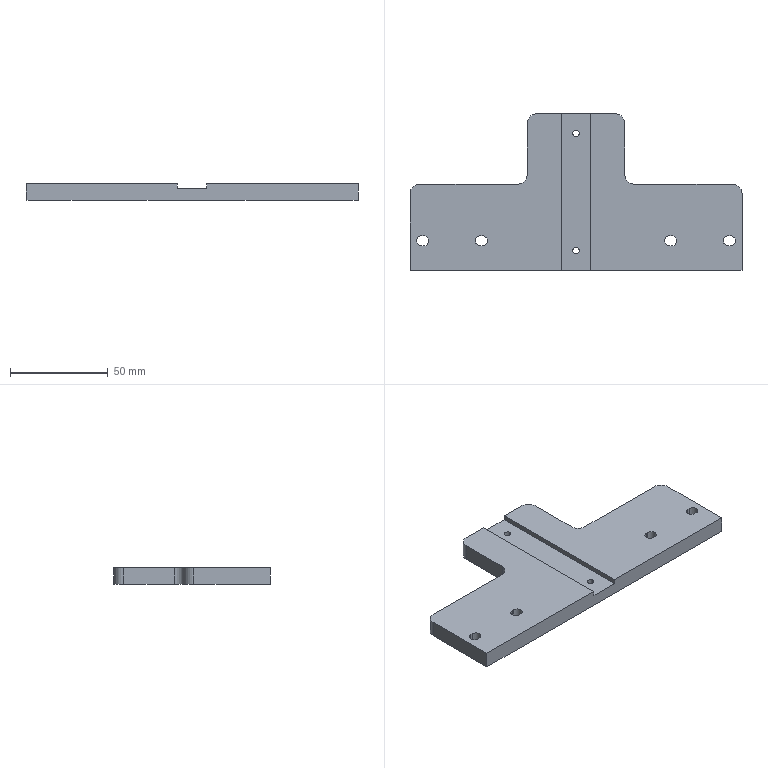Part | 1 solid | 44 faces | box 170 x 80 x 8.5 mm | volume 74787 mm3 | cylinder 22 | plane 22 | commonest cylinder face diameters 5.2 x12 10 x6 3.3 x4
STEP:
#1=CARTESIAN_POINT('',(1.65,-30.,0.));
#2=VERTEX_POINT('',#1);
#3=CARTESIAN_POINT('',(-1.65,-30.,0.));
#4=VERTEX_POINT('',#3);
#5=CARTESIAN_POINT('',(0.,-30.,0.));
#6=DIRECTION('',(0.,0.,-1.));
#7=DIRECTION('',(-1.,0.,0.));
#8=AXIS2_PLACEMENT_3D('',#5,#6,#7);
#9=CIRCLE('',#8,1.65);
#10=EDGE_CURVE('',#2,#4,#9,.T.);
#11=ORIENTED_EDGE('',*,*,#10,.T.);
#12=CARTESIAN_POINT('',(-1.65,-30.,6.));
#13=VERTEX_POINT('',#12);
#14=CARTESIAN_POINT('',(-1.65,-30.,8.5));
#15=DIRECTION('',(0.,0.,1.));
#16=VECTOR('',#15,1000.);
#17=LINE('',#14,#16);
#18=EDGE_CURVE('',#4,#13,#17,.T.);
#19=ORIENTED_EDGE('',*,*,#18,.T.);
#20=CARTESIAN_POINT('',(1.65,-30.,6.));
#21=VERTEX_POINT('',#20);
#22=CARTESIAN_POINT('',(0.,-30.,6.));
#23=DIRECTION('',(0.,0.,1.));
#24=DIRECTION('',(-1.,0.,0.));
#25=AXIS2_PLACEMENT_3D('',#22,#23,#24);
#26=CIRCLE('',#25,1.65);
#27=EDGE_CURVE('',#13,#21,#26,.T.);
#28=ORIENTED_EDGE('',*,*,#27,.T.);
#29=CARTESIAN_POINT('',(1.65,-30.,8.5));
#30=DIRECTION('',(0.,0.,1.));
#31=VECTOR('',#30,1000.);
#32=LINE('',#29,#31);
#33=EDGE_CURVE('',#2,#21,#32,.T.);
#34=ORIENTED_EDGE('',*,*,#33,.F.);
#35=EDGE_LOOP('',(#11,#19,#28,#34));
#36=FACE_OUTER_BOUND('',#35,.T.);
#37=CARTESIAN_POINT('',(0.,-30.,8.5));
#38=DIRECTION('',(0.,0.,1.));
#39=DIRECTION('',(1.,0.,0.));
#40=AXIS2_PLACEMENT_3D('',#37,#38,#39);
#41=CYLINDRICAL_SURFACE('',#40,1.65);
#42=ADVANCED_FACE('',(#36),#41,.F.);
#43=CARTESIAN_POINT('',(1.65,30.,0.));
#44=VERTEX_POINT('',#43);
#45=CARTESIAN_POINT('',(-1.65,30.,0.));
#46=VERTEX_POINT('',#45);
#47=CARTESIAN_POINT('',(0.,30.,0.));
#48=DIRECTION('',(0.,0.,-1.));
#49=DIRECTION('',(-1.,0.,0.));
#50=AXIS2_PLACEMENT_3D('',#47,#48,#49);
#51=CIRCLE('',#50,1.65);
#52=EDGE_CURVE('',#44,#46,#51,.T.);
#53=ORIENTED_EDGE('',*,*,#52,.T.);
#54=CARTESIAN_POINT('',(-1.65,30.,6.));
#55=VERTEX_POINT('',#54);
#56=CARTESIAN_POINT('',(-1.65,30.,8.5));
#57=DIRECTION('',(0.,0.,1.));
#58=VECTOR('',#57,1000.);
#59=LINE('',#56,#58);
#60=EDGE_CURVE('',#46,#55,#59,.T.);
#61=ORIENTED_EDGE('',*,*,#60,.T.);
#62=CARTESIAN_POINT('',(1.65,30.,6.));
#63=VERTEX_POINT('',#62);
#64=CARTESIAN_POINT('',(0.,30.,6.));
#65=DIRECTION('',(0.,0.,1.));
#66=DIRECTION('',(-1.,0.,0.));
#67=AXIS2_PLACEMENT_3D('',#64,#65,#66);
#68=CIRCLE('',#67,1.65);
#69=EDGE_CURVE('',#55,#63,#68,.T.);
#70=ORIENTED_EDGE('',*,*,#69,.T.);
#71=CARTESIAN_POINT('',(1.65,30.,8.5));
#72=DIRECTION('',(0.,0.,1.));
#73=VECTOR('',#72,1000.);
#74=LINE('',#71,#73);
#75=EDGE_CURVE('',#44,#63,#74,.T.);
#76=ORIENTED_EDGE('',*,*,#75,.F.);
#77=EDGE_LOOP('',(#53,#61,#70,#76));
#78=FACE_OUTER_BOUND('',#77,.T.);
#79=CARTESIAN_POINT('',(0.,30.,8.5));
#80=DIRECTION('',(0.,0.,1.));
#81=DIRECTION('',(1.,0.,0.));
#82=AXIS2_PLACEMENT_3D('',#79,#80,#81);
#83=CYLINDRICAL_SURFACE('',#82,1.65);
#84=ADVANCED_FACE('',(#78),#83,.F.);
#85=CARTESIAN_POINT('',(78.,-22.4,8.5));
#86=VERTEX_POINT('',#85);
#87=CARTESIAN_POINT('',(75.4,-25.,8.5));
#88=VERTEX_POINT('',#87);
#89=CARTESIAN_POINT('',(78.,-25.,8.5));
#90=DIRECTION('',(0.,0.,1.));
#91=DIRECTION('',(1.,0.,0.));
#92=AXIS2_PLACEMENT_3D('',#89,#90,#91);
#93=CIRCLE('',#92,2.6);
#94=EDGE_CURVE('',#86,#88,#93,.T.);
#95=ORIENTED_EDGE('',*,*,#94,.T.);
#96=CARTESIAN_POINT('',(75.4,-25.,0.));
#97=VERTEX_POINT('',#96);
#98=CARTESIAN_POINT('',(75.4,-25.,8.5));
#99=DIRECTION('',(0.,0.,-1.));
#100=VECTOR('',#99,1000.);
#101=LINE('',#98,#100);
#102=EDGE_CURVE('',#88,#97,#101,.T.);
#103=ORIENTED_EDGE('',*,*,#102,.T.);
#104=CARTESIAN_POINT('',(78.,-22.4,0.));
#105=VERTEX_POINT('',#104);
#106=CARTESIAN_POINT('',(78.,-25.,0.));
#107=DIRECTION('',(0.,0.,1.));
#108=DIRECTION('',(1.,0.,0.));
#109=AXIS2_PLACEMENT_3D('',#106,#107,#108);
#110=CIRCLE('',#109,2.6);
#111=EDGE_CURVE('',#105,#97,#110,.T.);
#112=ORIENTED_EDGE('',*,*,#111,.F.);
#113=CARTESIAN_POINT('',(78.,-22.4,8.5));
#114=DIRECTION('',(0.,0.,-1.));
#115=VECTOR('',#114,1000.);
#116=LINE('',#113,#115);
#117=EDGE_CURVE('',#86,#105,#116,.T.);
#118=ORIENTED_EDGE('',*,*,#117,.F.);
#119=EDGE_LOOP('',(#95,#103,#112,#118));
#120=FACE_OUTER_BOUND('',#119,.T.);
#121=CARTESIAN_POINT('',(78.,-25.,8.5));
#122=DIRECTION('',(0.,0.,-1.));
#123=DIRECTION('',(-1.,0.,0.));
#124=AXIS2_PLACEMENT_3D('',#121,#122,#123);
#125=CYLINDRICAL_SURFACE('',#124,2.6);
#126=ADVANCED_FACE('',(#120),#125,.F.);
#127=CARTESIAN_POINT('',(48.,-22.4,8.5));
#128=VERTEX_POINT('',#127);
#129=CARTESIAN_POINT('',(45.4,-25.,8.5));
#130=VERTEX_POINT('',#129);
#131=CARTESIAN_POINT('',(48.,-25.,8.5));
#132=DIRECTION('',(0.,0.,1.));
#133=DIRECTION('',(1.,0.,0.));
#134=AXIS2_PLACEMENT_3D('',#131,#132,#133);
#135=CIRCLE('',#134,2.6);
#136=EDGE_CURVE('',#128,#130,#135,.T.);
#137=ORIENTED_EDGE('',*,*,#136,.T.);
#138=CARTESIAN_POINT('',(45.4,-25.,0.));
#139=VERTEX_POINT('',#138);
#140=CARTESIAN_POINT('',(45.4,-25.,8.5));
#141=DIRECTION('',(0.,0.,-1.));
#142=VECTOR('',#141,1000.);
#143=LINE('',#140,#142);
#144=EDGE_CURVE('',#130,#139,#143,.T.);
#145=ORIENTED_EDGE('',*,*,#144,.T.);
#146=CARTESIAN_POINT('',(48.,-22.4,0.));
#147=VERTEX_POINT('',#146);
#148=CARTESIAN_POINT('',(48.,-25.,0.));
#149=DIRECTION('',(0.,0.,1.));
#150=DIRECTION('',(1.,0.,0.));
#151=AXIS2_PLACEMENT_3D('',#148,#149,#150);
#152=CIRCLE('',#151,2.6);
#153=EDGE_CURVE('',#147,#139,#152,.T.);
#154=ORIENTED_EDGE('',*,*,#153,.F.);
#155=CARTESIAN_POINT('',(48.,-22.4,8.5));
#156=DIRECTION('',(0.,0.,-1.));
#157=VECTOR('',#156,1000.);
#158=LINE('',#155,#157);
#159=EDGE_CURVE('',#128,#147,#158,.T.);
#160=ORIENTED_EDGE('',*,*,#159,.F.);
#161=EDGE_LOOP('',(#137,#145,#154,#160));
#162=FACE_OUTER_BOUND('',#161,.T.);
#163=CARTESIAN_POINT('',(48.,-25.,8.5));
#164=DIRECTION('',(0.,0.,-1.));
#165=DIRECTION('',(-1.,0.,0.));
#166=AXIS2_PLACEMENT_3D('',#163,#164,#165);
#167=CYLINDRICAL_SURFACE('',#166,2.6);
#168=ADVANCED_FACE('',(#162),#167,.F.);
#169=CARTESIAN_POINT('',(-49.,-22.4,8.5));
#170=VERTEX_POINT('',#169);
#171=CARTESIAN_POINT('',(-51.6,-25.,8.5));
#172=VERTEX_POINT('',#171);
#173=CARTESIAN_POINT('',(-49.,-25.,8.5));
#174=DIRECTION('',(0.,0.,1.));
#175=DIRECTION('',(1.,0.,0.));
#176=AXIS2_PLACEMENT_3D('',#173,#174,#175);
#177=CIRCLE('',#176,2.6);
#178=EDGE_CURVE('',#170,#172,#177,.T.);
#179=ORIENTED_EDGE('',*,*,#178,.T.);
#180=CARTESIAN_POINT('',(-51.6,-25.,0.));
#181=VERTEX_POINT('',#180);
#182=CARTESIAN_POINT('',(-51.6,-25.,8.5));
#183=DIRECTION('',(0.,0.,-1.));
#184=VECTOR('',#183,1000.);
#185=LINE('',#182,#184);
#186=EDGE_CURVE('',#172,#181,#185,.T.);
#187=ORIENTED_EDGE('',*,*,#186,.T.);
#188=CARTESIAN_POINT('',(-49.,-22.4,0.));
#189=VERTEX_POINT('',#188);
#190=CARTESIAN_POINT('',(-49.,-25.,0.));
#191=DIRECTION('',(0.,0.,1.));
#192=DIRECTION('',(1.,0.,0.));
#193=AXIS2_PLACEMENT_3D('',#190,#191,#192);
#194=CIRCLE('',#193,2.6);
#195=EDGE_CURVE('',#189,#181,#194,.T.);
#196=ORIENTED_EDGE('',*,*,#195,.F.);
#197=CARTESIAN_POINT('',(-49.,-22.4,8.5));
#198=DIRECTION('',(0.,0.,-1.));
#199=VECTOR('',#198,1000.);
#200=LINE('',#197,#199);
#201=EDGE_CURVE('',#170,#189,#200,.T.);
#202=ORIENTED_EDGE('',*,*,#201,.F.);
#203=EDGE_LOOP('',(#179,#187,#196,#202));
#204=FACE_OUTER_BOUND('',#203,.T.);
#205=CARTESIAN_POINT('',(-49.,-25.,8.5));
#206=DIRECTION('',(0.,0.,-1.));
#207=DIRECTION('',(-1.,0.,0.));
#208=AXIS2_PLACEMENT_3D('',#205,#206,#207);
#209=CYLINDRICAL_SURFACE('',#208,2.6);
#210=ADVANCED_FACE('',(#204),#209,.F.);
#211=CARTESIAN_POINT('',(-79.,-22.4,8.5));
#212=VERTEX_POINT('',#211);
#213=CARTESIAN_POINT('',(-81.6,-25.,8.5));
#214=VERTEX_POINT('',#213);
#215=CARTESIAN_POINT('',(-79.,-25.,8.5));
#216=DIRECTION('',(0.,0.,1.));
#217=DIRECTION('',(1.,0.,0.));
#218=AXIS2_PLACEMENT_3D('',#215,#216,#217);
#219=CIRCLE('',#218,2.6);
#220=EDGE_CURVE('',#212,#214,#219,.T.);
#221=ORIENTED_EDGE('',*,*,#220,.T.);
#222=CARTESIAN_POINT('',(-81.6,-25.,0.));
#223=VERTEX_POINT('',#222);
#224=CARTESIAN_POINT('',(-81.6,-25.,8.5));
#225=DIRECTION('',(0.,0.,-1.));
#226=VECTOR('',#225,1000.);
#227=LINE('',#224,#226);
#228=EDGE_CURVE('',#214,#223,#227,.T.);
#229=ORIENTED_EDGE('',*,*,#228,.T.);
#230=CARTESIAN_POINT('',(-79.,-22.4,0.));
#231=VERTEX_POINT('',#230);
#232=CARTESIAN_POINT('',(-79.,-25.,0.));
#233=DIRECTION('',(0.,0.,1.));
#234=DIRECTION('',(1.,0.,0.));
#235=AXIS2_PLACEMENT_3D('',#232,#233,#234);
#236=CIRCLE('',#235,2.6);
#237=EDGE_CURVE('',#231,#223,#236,.T.);
#238=ORIENTED_EDGE('',*,*,#237,.F.);
#239=CARTESIAN_POINT('',(-79.,-22.4,8.5));
#240=DIRECTION('',(0.,0.,-1.));
#241=VECTOR('',#240,1000.);
#242=LINE('',#239,#241);
#243=EDGE_CURVE('',#212,#231,#242,.T.);
#244=ORIENTED_EDGE('',*,*,#243,.F.);
#245=EDGE_LOOP('',(#221,#229,#238,#244));
#246=FACE_OUTER_BOUND('',#245,.T.);
#247=CARTESIAN_POINT('',(-79.,-25.,8.5));
#248=DIRECTION('',(0.,0.,-1.));
#249=DIRECTION('',(-1.,0.,0.));
#250=AXIS2_PLACEMENT_3D('',#247,#248,#249);
#251=CYLINDRICAL_SURFACE('',#250,2.6);
#252=ADVANCED_FACE('',(#246),#251,.F.);
#253=ORIENTED_EDGE('',*,*,#178,.F.);
#254=CARTESIAN_POINT('',(-48.,-22.4,8.5));
#255=VERTEX_POINT('',#254);
#256=CARTESIAN_POINT('',(-49.,-22.4,8.5));
#257=DIRECTION('',(-1.,0.,0.));
#258=VECTOR('',#257,1000.);
#259=LINE('',#256,#258);
#260=EDGE_CURVE('',#255,#170,#259,.T.);
#261=ORIENTED_EDGE('',*,*,#260,.F.);
#262=CARTESIAN_POINT('',(-48.,-27.6,8.5));
#263=VERTEX_POINT('',#262);
#264=CARTESIAN_POINT('',(-48.,-25.,8.5));
#265=DIRECTION('',(0.,0.,1.));
#266=DIRECTION('',(1.,0.,0.));
#267=AXIS2_PLACEMENT_3D('',#264,#265,#266);
#268=CIRCLE('',#267,2.6);
#269=EDGE_CURVE('',#263,#255,#268,.T.);
#270=ORIENTED_EDGE('',*,*,#269,.F.);
#271=CARTESIAN_POINT('',(-49.,-27.6,8.5));
#272=VERTEX_POINT('',#271);
#273=CARTESIAN_POINT('',(-49.,-27.6,8.5));
#274=DIRECTION('',(1.,0.,0.));
#275=VECTOR('',#274,1000.);
#276=LINE('',#273,#275);
#277=EDGE_CURVE('',#272,#263,#276,.T.);
#278=ORIENTED_EDGE('',*,*,#277,.F.);
#279=CARTESIAN_POINT('',(-49.,-25.,8.5));
#280=DIRECTION('',(0.,0.,1.));
#281=DIRECTION('',(1.,0.,0.));
#282=AXIS2_PLACEMENT_3D('',#279,#280,#281);
#283=CIRCLE('',#282,2.6);
#284=EDGE_CURVE('',#172,#272,#283,.T.);
#285=ORIENTED_EDGE('',*,*,#284,.F.);
#286=EDGE_LOOP('',(#253,#261,#270,#278,#285));
#287=FACE_BOUND('',#286,.T.);
#288=ORIENTED_EDGE('',*,*,#220,.F.);
#289=CARTESIAN_POINT('',(-78.,-22.4,8.5));
#290=VERTEX_POINT('',#289);
#291=CARTESIAN_POINT('',(-79.,-22.4,8.5));
#292=DIRECTION('',(-1.,0.,0.));
#293=VECTOR('',#292,1000.);
#294=LINE('',#291,#293);
#295=EDGE_CURVE('',#290,#212,#294,.T.);
#296=ORIENTED_EDGE('',*,*,#295,.F.);
#297=CARTESIAN_POINT('',(-78.,-27.6,8.5));
#298=VERTEX_POINT('',#297);
#299=CARTESIAN_POINT('',(-78.,-25.,8.5));
#300=DIRECTION('',(0.,0.,1.));
#301=DIRECTION('',(1.,0.,0.));
#302=AXIS2_PLACEMENT_3D('',#299,#300,#301);
#303=CIRCLE('',#302,2.6);
#304=EDGE_CURVE('',#298,#290,#303,.T.);
#305=ORIENTED_EDGE('',*,*,#304,.F.);
#306=CARTESIAN_POINT('',(-79.,-27.6,8.5));
#307=VERTEX_POINT('',#306);
#308=CARTESIAN_POINT('',(-79.,-27.6,8.5));
#309=DIRECTION('',(1.,0.,0.));
#310=VECTOR('',#309,1000.);
#311=LINE('',#308,#310);
#312=EDGE_CURVE('',#307,#298,#311,.T.);
#313=ORIENTED_EDGE('',*,*,#312,.F.);
#314=CARTESIAN_POINT('',(-79.,-25.,8.5));
#315=DIRECTION('',(0.,0.,1.));
#316=DIRECTION('',(1.,0.,0.));
#317=AXIS2_PLACEMENT_3D('',#314,#315,#316);
#318=CIRCLE('',#317,2.6);
#319=EDGE_CURVE('',#214,#307,#318,.T.);
#320=ORIENTED_EDGE('',*,*,#319,.F.);
#321=EDGE_LOOP('',(#288,#296,#305,#313,#320));
#322=FACE_BOUND('',#321,.T.);
#323=CARTESIAN_POINT('',(-85.,-40.,8.5));
#324=VERTEX_POINT('',#323);
#325=CARTESIAN_POINT('',(-7.5,-40.,8.5));
#326=VERTEX_POINT('',#325);
#327=CARTESIAN_POINT('',(-85.,-40.,8.5));
#328=DIRECTION('',(1.,0.,0.));
#329=VECTOR('',#328,1000.);
#330=LINE('',#327,#329);
#331=EDGE_CURVE('',#324,#326,#330,.T.);
#332=ORIENTED_EDGE('',*,*,#331,.T.);
#333=CARTESIAN_POINT('',(-7.5,40.,8.5));
#334=VERTEX_POINT('',#333);
#335=CARTESIAN_POINT('',(-7.5,40.,8.5));
#336=DIRECTION('',(0.,-1.,0.));
#337=VECTOR('',#336,1000.);
#338=LINE('',#335,#337);
#339=EDGE_CURVE('',#334,#326,#338,.T.);
#340=ORIENTED_EDGE('',*,*,#339,.F.);
#341=CARTESIAN_POINT('',(-20.,40.,8.5));
#342=VERTEX_POINT('',#341);
#343=CARTESIAN_POINT('',(-85.,40.,8.5));
#344=DIRECTION('',(-1.,0.,0.));
#345=VECTOR('',#344,1000.);
#346=LINE('',#343,#345);
#347=EDGE_CURVE('',#334,#342,#346,.T.);
#348=ORIENTED_EDGE('',*,*,#347,.T.);
#349=CARTESIAN_POINT('',(-25.,35.,8.5));
#350=VERTEX_POINT('',#349);
#351=CARTESIAN_POINT('',(-20.,35.,8.5));
#352=DIRECTION('',(0.,0.,1.));
#353=DIRECTION('',(-1.,0.,0.));
#354=AXIS2_PLACEMENT_3D('',#351,#352,#353);
#355=CIRCLE('',#354,5.);
#356=EDGE_CURVE('',#342,#350,#355,.T.);
#357=ORIENTED_EDGE('',*,*,#356,.T.);
#358=CARTESIAN_POINT('',(-25.,9.,8.5));
#359=VERTEX_POINT('',#358);
#360=CARTESIAN_POINT('',(-25.,40.,8.5));
#361=DIRECTION('',(0.,1.,0.));
#362=VECTOR('',#361,1000.);
#363=LINE('',#360,#362);
#364=EDGE_CURVE('',#359,#350,#363,.T.);
#365=ORIENTED_EDGE('',*,*,#364,.F.);
#366=CARTESIAN_POINT('',(-30.,4.,8.5));
#367=VERTEX_POINT('',#366);
#368=CARTESIAN_POINT('',(-30.,9.,8.5));
#369=DIRECTION('',(0.,0.,-1.));
#370=DIRECTION('',(-1.,0.,0.));
#371=AXIS2_PLACEMENT_3D('',#368,#369,#370);
#372=CIRCLE('',#371,5.);
#373=EDGE_CURVE('',#359,#367,#372,.T.);
#374=ORIENTED_EDGE('',*,*,#373,.T.);
#375=CARTESIAN_POINT('',(-80.,4.,8.5));
#376=VERTEX_POINT('',#375);
#377=CARTESIAN_POINT('',(-25.,4.,8.5));
#378=DIRECTION('',(1.,0.,0.));
#379=VECTOR('',#378,1000.);
#380=LINE('',#377,#379);
#381=EDGE_CURVE('',#376,#367,#380,.T.);
#382=ORIENTED_EDGE('',*,*,#381,.F.);
#383=CARTESIAN_POINT('',(-85.,-1.,8.5));
#384=VERTEX_POINT('',#383);
#385=CARTESIAN_POINT('',(-80.,-1.,8.5));
#386=DIRECTION('',(0.,0.,1.));
#387=DIRECTION('',(-1.,0.,0.));
#388=AXIS2_PLACEMENT_3D('',#385,#386,#387);
#389=CIRCLE('',#388,5.);
#390=EDGE_CURVE('',#376,#384,#389,.T.);
#391=ORIENTED_EDGE('',*,*,#390,.T.);
#392=CARTESIAN_POINT('',(-85.,-40.,8.5));
#393=DIRECTION('',(0.,-1.,0.));
#394=VECTOR('',#393,1000.);
#395=LINE('',#392,#394);
#396=EDGE_CURVE('',#384,#324,#395,.T.);
#397=ORIENTED_EDGE('',*,*,#396,.T.);
#398=EDGE_LOOP('',(#332,#340,#348,#357,#365,#374,#382,#391,#397));
#399=FACE_OUTER_BOUND('',#398,.T.);
#400=CARTESIAN_POINT('',(0.,0.,8.5));
#401=DIRECTION('',(0.,0.,-1.));
#402=DIRECTION('',(-1.,0.,0.));
#403=AXIS2_PLACEMENT_3D('',#400,#401,#402);
#404=PLANE('',#403);
#405=ADVANCED_FACE('',(#287,#322,#399),#404,.F.);
#406=CARTESIAN_POINT('',(20.,40.,8.5));
#407=VERTEX_POINT('',#406);
#408=CARTESIAN_POINT('',(7.5,40.,8.5));
#409=VERTEX_POINT('',#408);
#410=CARTESIAN_POINT('',(-85.,40.,8.5));
#411=DIRECTION('',(-1.,0.,0.));
#412=VECTOR('',#411,1000.);
#413=LINE('',#410,#412);
#414=EDGE_CURVE('',#407,#409,#413,.T.);
#415=ORIENTED_EDGE('',*,*,#414,.T.);
#416=CARTESIAN_POINT('',(7.5,-40.,8.5));
#417=VERTEX_POINT('',#416);
#418=CARTESIAN_POINT('',(7.5,40.,8.5));
#419=DIRECTION('',(0.,-1.,0.));
#420=VECTOR('',#419,1000.);
#421=LINE('',#418,#420);
#422=EDGE_CURVE('',#409,#417,#421,.T.);
#423=ORIENTED_EDGE('',*,*,#422,.T.);
#424=CARTESIAN_POINT('',(85.,-40.,8.5));
#425=VERTEX_POINT('',#424);
#426=CARTESIAN_POINT('',(-85.,-40.,8.5));
#427=DIRECTION('',(1.,0.,0.));
#428=VECTOR('',#427,1000.);
#429=LINE('',#426,#428);
#430=EDGE_CURVE('',#417,#425,#429,.T.);
#431=ORIENTED_EDGE('',*,*,#430,.T.);
#432=CARTESIAN_POINT('',(85.,-1.,8.5));
#433=VERTEX_POINT('',#432);
#434=CARTESIAN_POINT('',(85.,-40.,8.5));
#435=DIRECTION('',(0.,1.,0.));
#436=VECTOR('',#435,1000.);
#437=LINE('',#434,#436);
#438=EDGE_CURVE('',#425,#433,#437,.T.);
#439=ORIENTED_EDGE('',*,*,#438,.T.);
#440=CARTESIAN_POINT('',(80.,4.,8.5));
#441=VERTEX_POINT('',#440);
#442=CARTESIAN_POINT('',(80.,-1.,8.5));
#443=DIRECTION('',(0.,0.,1.));
#444=DIRECTION('',(-1.,0.,0.));
#445=AXIS2_PLACEMENT_3D('',#442,#443,#444);
#446=CIRCLE('',#445,5.);
#447=EDGE_CURVE('',#433,#441,#446,.T.);
#448=ORIENTED_EDGE('',*,*,#447,.T.);
#449=CARTESIAN_POINT('',(30.,4.,8.5));
#450=VERTEX_POINT('',#449);
#451=CARTESIAN_POINT('',(25.,4.,8.5));
#452=DIRECTION('',(-1.,0.,0.));
#453=VECTOR('',#452,1000.);
#454=LINE('',#451,#453);
#455=EDGE_CURVE('',#441,#450,#454,.T.);
#456=ORIENTED_EDGE('',*,*,#455,.T.);
#457=CARTESIAN_POINT('',(25.,9.,8.5));
#458=VERTEX_POINT('',#457);
#459=CARTESIAN_POINT('',(30.,9.,8.5));
#460=DIRECTION('',(0.,0.,-1.));
#461=DIRECTION('',(-1.,0.,0.));
#462=AXIS2_PLACEMENT_3D('',#459,#460,#461);
#463=CIRCLE('',#462,5.);
#464=EDGE_CURVE('',#450,#458,#463,.T.);
#465=ORIENTED_EDGE('',*,*,#464,.T.);
#466=CARTESIAN_POINT('',(25.,35.,8.5));
#467=VERTEX_POINT('',#466);
#468=CARTESIAN_POINT('',(25.,40.,8.5));
#469=DIRECTION('',(0.,1.,0.));
#470=VECTOR('',#469,1000.);
#471=LINE('',#468,#470);
#472=EDGE_CURVE('',#458,#467,#471,.T.);
#473=ORIENTED_EDGE('',*,*,#472,.T.);
#474=CARTESIAN_POINT('',(20.,35.,8.5));
#475=DIRECTION('',(0.,0.,1.));
#476=DIRECTION('',(-1.,0.,0.));
#477=AXIS2_PLACEMENT_3D('',#474,#475,#476);
#478=CIRCLE('',#477,5.);
#479=EDGE_CURVE('',#467,#407,#478,.T.);
#480=ORIENTED_EDGE('',*,*,#479,.T.);
#481=EDGE_LOOP('',(#415,#423,#431,#439,#448,#456,#465,#473,#480));
#482=FACE_OUTER_BOUND('',#481,.T.);
#483=ORIENTED_EDGE('',*,*,#136,.F.);
#484=CARTESIAN_POINT('',(49.,-22.4,8.5));
#485=VERTEX_POINT('',#484);
#486=CARTESIAN_POINT('',(48.,-22.4,8.5));
#487=DIRECTION('',(-1.,0.,0.));
#488=VECTOR('',#487,1000.);
#489=LINE('',#486,#488);
#490=EDGE_CURVE('',#485,#128,#489,.T.);
#491=ORIENTED_EDGE('',*,*,#490,.F.);
#492=CARTESIAN_POINT('',(49.,-27.6,8.5));
#493=VERTEX_POINT('',#492);
#494=CARTESIAN_POINT('',(49.,-25.,8.5));
#495=DIRECTION('',(0.,0.,1.));
#496=DIRECTION('',(1.,0.,0.));
#497=AXIS2_PLACEMENT_3D('',#494,#495,#496);
#498=CIRCLE('',#497,2.6);
#499=EDGE_CURVE('',#493,#485,#498,.T.);
#500=ORIENTED_EDGE('',*,*,#499,.F.);
#501=CARTESIAN_POINT('',(48.,-27.6,8.5));
#502=VERTEX_POINT('',#501);
#503=CARTESIAN_POINT('',(48.,-27.6,8.5));
#504=DIRECTION('',(1.,0.,0.));
#505=VECTOR('',#504,1000.);
#506=LINE('',#503,#505);
#507=EDGE_CURVE('',#502,#493,#506,.T.);
#508=ORIENTED_EDGE('',*,*,#507,.F.);
#509=CARTESIAN_POINT('',(48.,-25.,8.5));
#510=DIRECTION('',(0.,0.,1.));
#511=DIRECTION('',(1.,0.,0.));
#512=AXIS2_PLACEMENT_3D('',#509,#510,#511);
#513=CIRCLE('',#512,2.6);
#514=EDGE_CURVE('',#130,#502,#513,.T.);
#515=ORIENTED_EDGE('',*,*,#514,.F.);
#516=EDGE_LOOP('',(#483,#491,#500,#508,#515));
#517=FACE_BOUND('',#516,.T.);
#518=ORIENTED_EDGE('',*,*,#94,.F.);
#519=CARTESIAN_POINT('',(79.,-22.4,8.5));
#520=VERTEX_POINT('',#519);
#521=CARTESIAN_POINT('',(78.,-22.4,8.5));
#522=DIRECTION('',(-1.,0.,0.));
#523=VECTOR('',#522,1000.);
#524=LINE('',#521,#523);
#525=EDGE_CURVE('',#520,#86,#524,.T.);
#526=ORIENTED_EDGE('',*,*,#525,.F.);
#527=CARTESIAN_POINT('',(79.,-27.6,8.5));
#528=VERTEX_POINT('',#527);
#529=CARTESIAN_POINT('',(79.,-25.,8.5));
#530=DIRECTION('',(0.,0.,1.));
#531=DIRECTION('',(1.,0.,0.));
#532=AXIS2_PLACEMENT_3D('',#529,#530,#531);
#533=CIRCLE('',#532,2.6);
#534=EDGE_CURVE('',#528,#520,#533,.T.);
#535=ORIENTED_EDGE('',*,*,#534,.F.);
#536=CARTESIAN_POINT('',(78.,-27.6,8.5));
#537=VERTEX_POINT('',#536);
#538=CARTESIAN_POINT('',(78.,-27.6,8.5));
#539=DIRECTION('',(1.,0.,0.));
#540=VECTOR('',#539,1000.);
#541=LINE('',#538,#540);
#542=EDGE_CURVE('',#537,#528,#541,.T.);
#543=ORIENTED_EDGE('',*,*,#542,.F.);
#544=CARTESIAN_POINT('',(78.,-25.,8.5));
#545=DIRECTION('',(0.,0.,1.));
#546=DIRECTION('',(1.,0.,0.));
#547=AXIS2_PLACEMENT_3D('',#544,#545,#546);
#548=CIRCLE('',#547,2.6);
#549=EDGE_CURVE('',#88,#537,#548,.T.);
#550=ORIENTED_EDGE('',*,*,#549,.F.);
#551=EDGE_LOOP('',(#518,#526,#535,#543,#550));
#552=FACE_BOUND('',#551,.T.);
#553=CARTESIAN_POINT('',(0.,0.,8.5));
#554=DIRECTION('',(0.,0.,-1.));
#555=DIRECTION('',(-1.,0.,0.));
#556=AXIS2_PLACEMENT_3D('',#553,#554,#555);
#557=PLANE('',#556);
#558=ADVANCED_FACE('',(#482,#517,#552),#557,.F.);
#559=ORIENTED_EDGE('',*,*,#10,.F.);
#560=CARTESIAN_POINT('',(0.,-30.,0.));
#561=DIRECTION('',(0.,0.,-1.));
#562=DIRECTION('',(-1.,0.,0.));
#563=AXIS2_PLACEMENT_3D('',#560,#561,#562);
#564=CIRCLE('',#563,1.65);
#565=EDGE_CURVE('',#4,#2,#564,.T.);
#566=ORIENTED_EDGE('',*,*,#565,.F.);
#567=EDGE_LOOP('',(#559,#566));
#568=FACE_BOUND('',#567,.T.);
#569=ORIENTED_EDGE('',*,*,#52,.F.);
#570=CARTESIAN_POINT('',(0.,30.,0.));
#571=DIRECTION('',(0.,0.,-1.));
#572=DIRECTION('',(-1.,0.,0.));
#573=AXIS2_PLACEMENT_3D('',#570,#571,#572);
#574=CIRCLE('',#573,1.65);
#575=EDGE_CURVE('',#46,#44,#574,.T.);
#576=ORIENTED_EDGE('',*,*,#575,.F.);
#577=EDGE_LOOP('',(#569,#576));
#578=FACE_BOUND('',#577,.T.);
#579=CARTESIAN_POINT('',(-78.,-22.4,0.));
#580=VERTEX_POINT('',#579);
#581=CARTESIAN_POINT('',(-79.,-22.4,0.));
#582=DIRECTION('',(-1.,0.,0.));
#583=VECTOR('',#582,1000.);
#584=LINE('',#581,#583);
#585=EDGE_CURVE('',#580,#231,#584,.T.);
#586=ORIENTED_EDGE('',*,*,#585,.T.);
#587=ORIENTED_EDGE('',*,*,#237,.T.);
#588=CARTESIAN_POINT('',(-79.,-27.6,0.));
#589=VERTEX_POINT('',#588);
#590=CARTESIAN_POINT('',(-79.,-25.,0.));
#591=DIRECTION('',(0.,0.,1.));
#592=DIRECTION('',(1.,0.,0.));
#593=AXIS2_PLACEMENT_3D('',#590,#591,#592);
#594=CIRCLE('',#593,2.6);
#595=EDGE_CURVE('',#223,#589,#594,.T.);
#596=ORIENTED_EDGE('',*,*,#595,.T.);
#597=CARTESIAN_POINT('',(-78.,-27.6,0.));
#598=VERTEX_POINT('',#597);
#599=CARTESIAN_POINT('',(-79.,-27.6,0.));
#600=DIRECTION('',(1.,0.,0.));
#601=VECTOR('',#600,1000.);
#602=LINE('',#599,#601);
#603=EDGE_CURVE('',#589,#598,#602,.T.);
#604=ORIENTED_EDGE('',*,*,#603,.T.);
#605=CARTESIAN_POINT('',(-78.,-25.,0.));
#606=DIRECTION('',(0.,0.,1.));
#607=DIRECTION('',(1.,0.,0.));
#608=AXIS2_PLACEMENT_3D('',#605,#606,#607);
#609=CIRCLE('',#608,2.6);
#610=EDGE_CURVE('',#598,#580,#609,.T.);
#611=ORIENTED_EDGE('',*,*,#610,.T.);
#612=EDGE_LOOP('',(#586,#587,#596,#604,#611));
#613=FACE_BOUND('',#612,.T.);
#614=CARTESIAN_POINT('',(-48.,-22.4,0.));
#615=VERTEX_POINT('',#614);
#616=CARTESIAN_POINT('',(-49.,-22.4,0.));
#617=DIRECTION('',(-1.,0.,0.));
#618=VECTOR('',#617,1000.);
#619=LINE('',#616,#618);
#620=EDGE_CURVE('',#615,#189,#619,.T.);
#621=ORIENTED_EDGE('',*,*,#620,.T.);
#622=ORIENTED_EDGE('',*,*,#195,.T.);
#623=CARTESIAN_POINT('',(-49.,-27.6,0.));
#624=VERTEX_POINT('',#623);
#625=CARTESIAN_POINT('',(-49.,-25.,0.));
#626=DIRECTION('',(0.,0.,1.));
#627=DIRECTION('',(1.,0.,0.));
#628=AXIS2_PLACEMENT_3D('',#625,#626,#627);
#629=CIRCLE('',#628,2.6);
#630=EDGE_CURVE('',#181,#624,#629,.T.);
#631=ORIENTED_EDGE('',*,*,#630,.T.);
#632=CARTESIAN_POINT('',(-48.,-27.6,0.));
#633=VERTEX_POINT('',#632);
#634=CARTESIAN_POINT('',(-49.,-27.6,0.));
#635=DIRECTION('',(1.,0.,0.));
#636=VECTOR('',#635,1000.);
#637=LINE('',#634,#636);
#638=EDGE_CURVE('',#624,#633,#637,.T.);
#639=ORIENTED_EDGE('',*,*,#638,.T.);
#640=CARTESIAN_POINT('',(-48.,-25.,0.));
#641=DIRECTION('',(0.,0.,1.));
#642=DIRECTION('',(1.,0.,0.));
#643=AXIS2_PLACEMENT_3D('',#640,#641,#642);
#644=CIRCLE('',#643,2.6);
#645=EDGE_CURVE('',#633,#615,#644,.T.);
#646=ORIENTED_EDGE('',*,*,#645,.T.);
#647=EDGE_LOOP('',(#621,#622,#631,#639,#646));
#648=FACE_BOUND('',#647,.T.);
#649=CARTESIAN_POINT('',(49.,-22.4,0.));
#650=VERTEX_POINT('',#649);
#651=CARTESIAN_POINT('',(48.,-22.4,0.));
#652=DIRECTION('',(-1.,0.,0.));
#653=VECTOR('',#652,1000.);
#654=LINE('',#651,#653);
#655=EDGE_CURVE('',#650,#147,#654,.T.);
#656=ORIENTED_EDGE('',*,*,#655,.T.);
#657=ORIENTED_EDGE('',*,*,#153,.T.);
#658=CARTESIAN_POINT('',(48.,-27.6,0.));
#659=VERTEX_POINT('',#658);
#660=CARTESIAN_POINT('',(48.,-25.,0.));
#661=DIRECTION('',(0.,0.,1.));
#662=DIRECTION('',(1.,0.,0.));
#663=AXIS2_PLACEMENT_3D('',#660,#661,#662);
#664=CIRCLE('',#663,2.6);
#665=EDGE_CURVE('',#139,#659,#664,.T.);
#666=ORIENTED_EDGE('',*,*,#665,.T.);
#667=CARTESIAN_POINT('',(49.,-27.6,0.));
#668=VERTEX_POINT('',#667);
#669=CARTESIAN_POINT('',(48.,-27.6,0.));
#670=DIRECTION('',(1.,0.,0.));
#671=VECTOR('',#670,1000.);
#672=LINE('',#669,#671);
#673=EDGE_CURVE('',#659,#668,#672,.T.);
#674=ORIENTED_EDGE('',*,*,#673,.T.);
#675=CARTESIAN_POINT('',(49.,-25.,0.));
#676=DIRECTION('',(0.,0.,1.));
#677=DIRECTION('',(1.,0.,0.));
#678=AXIS2_PLACEMENT_3D('',#675,#676,#677);
#679=CIRCLE('',#678,2.6);
#680=EDGE_CURVE('',#668,#650,#679,.T.);
#681=ORIENTED_EDGE('',*,*,#680,.T.);
#682=EDGE_LOOP('',(#656,#657,#666,#674,#681));
#683=FACE_BOUND('',#682,.T.);
#684=CARTESIAN_POINT('',(79.,-22.4,0.));
#685=VERTEX_POINT('',#684);
#686=CARTESIAN_POINT('',(78.,-22.4,0.));
#687=DIRECTION('',(-1.,0.,0.));
#688=VECTOR('',#687,1000.);
#689=LINE('',#686,#688);
#690=EDGE_CURVE('',#685,#105,#689,.T.);
#691=ORIENTED_EDGE('',*,*,#690,.T.);
#692=ORIENTED_EDGE('',*,*,#111,.T.);
#693=CARTESIAN_POINT('',(78.,-27.6,0.));
#694=VERTEX_POINT('',#693);
#695=CARTESIAN_POINT('',(78.,-25.,0.));
#696=DIRECTION('',(0.,0.,1.));
#697=DIRECTION('',(1.,0.,0.));
#698=AXIS2_PLACEMENT_3D('',#695,#696,#697);
#699=CIRCLE('',#698,2.6);
#700=EDGE_CURVE('',#97,#694,#699,.T.);
#701=ORIENTED_EDGE('',*,*,#700,.T.);
#702=CARTESIAN_POINT('',(79.,-27.6,0.));
#703=VERTEX_POINT('',#702);
#704=CARTESIAN_POINT('',(78.,-27.6,0.));
#705=DIRECTION('',(1.,0.,0.));
#706=VECTOR('',#705,1000.);
#707=LINE('',#704,#706);
#708=EDGE_CURVE('',#694,#703,#707,.T.);
#709=ORIENTED_EDGE('',*,*,#708,.T.);
#710=CARTESIAN_POINT('',(79.,-25.,0.));
#711=DIRECTION('',(0.,0.,1.));
#712=DIRECTION('',(1.,0.,0.));
#713=AXIS2_PLACEMENT_3D('',#710,#711,#712);
#714=CIRCLE('',#713,2.6);
#715=EDGE_CURVE('',#703,#685,#714,.T.);
#716=ORIENTED_EDGE('',*,*,#715,.T.);
#717=EDGE_LOOP('',(#691,#692,#701,#709,#716));
#718=FACE_BOUND('',#717,.T.);
#719=CARTESIAN_POINT('',(-85.,-1.,0.));
#720=VERTEX_POINT('',#719);
#721=CARTESIAN_POINT('',(-85.,-40.,0.));
#722=VERTEX_POINT('',#721);
#723=CARTESIAN_POINT('',(-85.,-40.,0.));
#724=DIRECTION('',(0.,-1.,0.));
#725=VECTOR('',#724,1000.);
#726=LINE('',#723,#725);
#727=EDGE_CURVE('',#720,#722,#726,.T.);
#728=ORIENTED_EDGE('',*,*,#727,.F.);
#729=CARTESIAN_POINT('',(-80.,4.,0.));
#730=VERTEX_POINT('',#729);
#731=CARTESIAN_POINT('',(-80.,-1.,0.));
#732=DIRECTION('',(0.,0.,-1.));
#733=DIRECTION('',(-1.,0.,0.));
#734=AXIS2_PLACEMENT_3D('',#731,#732,#733);
#735=CIRCLE('',#734,5.);
#736=EDGE_CURVE('',#720,#730,#735,.T.);
#737=ORIENTED_EDGE('',*,*,#736,.T.);
#738=CARTESIAN_POINT('',(-30.,4.,0.));
#739=VERTEX_POINT('',#738);
#740=CARTESIAN_POINT('',(0.,4.,0.));
#741=DIRECTION('',(-1.,0.,0.));
#742=VECTOR('',#741,1000.);
#743=LINE('',#740,#742);
#744=EDGE_CURVE('',#739,#730,#743,.T.);
#745=ORIENTED_EDGE('',*,*,#744,.F.);
#746=CARTESIAN_POINT('',(-25.,9.,0.));
#747=VERTEX_POINT('',#746);
#748=CARTESIAN_POINT('',(-30.,9.,0.));
#749=DIRECTION('',(0.,0.,1.));
#750=DIRECTION('',(-1.,0.,0.));
#751=AXIS2_PLACEMENT_3D('',#748,#749,#750);
#752=CIRCLE('',#751,5.);
#753=EDGE_CURVE('',#739,#747,#752,.T.);
#754=ORIENTED_EDGE('',*,*,#753,.T.);
#755=CARTESIAN_POINT('',(-25.,35.,0.));
#756=VERTEX_POINT('',#755);
#757=CARTESIAN_POINT('',(-25.,0.,0.));
#758=DIRECTION('',(0.,-1.,0.));
#759=VECTOR('',#758,1000.);
#760=LINE('',#757,#759);
#761=EDGE_CURVE('',#756,#747,#760,.T.);
#762=ORIENTED_EDGE('',*,*,#761,.F.);
#763=CARTESIAN_POINT('',(-20.,40.,0.));
#764=VERTEX_POINT('',#763);
#765=CARTESIAN_POINT('',(-20.,35.,0.));
#766=DIRECTION('',(0.,0.,-1.));
#767=DIRECTION('',(-1.,0.,0.));
#768=AXIS2_PLACEMENT_3D('',#765,#766,#767);
#769=CIRCLE('',#768,5.);
#770=EDGE_CURVE('',#756,#764,#769,.T.);
#771=ORIENTED_EDGE('',*,*,#770,.T.);
#772=CARTESIAN_POINT('',(20.,40.,0.));
#773=VERTEX_POINT('',#772);
#774=CARTESIAN_POINT('',(-85.,40.,0.));
#775=DIRECTION('',(-1.,0.,0.));
#776=VECTOR('',#775,1000.);
#777=LINE('',#774,#776);
#778=EDGE_CURVE('',#773,#764,#777,.T.);
#779=ORIENTED_EDGE('',*,*,#778,.F.);
#780=CARTESIAN_POINT('',(25.,35.,0.));
#781=VERTEX_POINT('',#780);
#782=CARTESIAN_POINT('',(20.,35.,0.));
#783=DIRECTION('',(0.,0.,-1.));
#784=DIRECTION('',(-1.,0.,0.));
#785=AXIS2_PLACEMENT_3D('',#782,#783,#784);
#786=CIRCLE('',#785,5.);
#787=EDGE_CURVE('',#773,#781,#786,.T.);
#788=ORIENTED_EDGE('',*,*,#787,.T.);
#789=CARTESIAN_POINT('',(25.,9.,0.));
#790=VERTEX_POINT('',#789);
#791=CARTESIAN_POINT('',(25.,0.,0.));
#792=DIRECTION('',(0.,-1.,0.));
#793=VECTOR('',#792,1000.);
#794=LINE('',#791,#793);
#795=EDGE_CURVE('',#781,#790,#794,.T.);
#796=ORIENTED_EDGE('',*,*,#795,.T.);
#797=CARTESIAN_POINT('',(30.,4.,0.));
#798=VERTEX_POINT('',#797);
#799=CARTESIAN_POINT('',(30.,9.,0.));
#800=DIRECTION('',(0.,0.,1.));
#801=DIRECTION('',(-1.,0.,0.));
#802=AXIS2_PLACEMENT_3D('',#799,#800,#801);
#803=CIRCLE('',#802,5.);
#804=EDGE_CURVE('',#790,#798,#803,.T.);
#805=ORIENTED_EDGE('',*,*,#804,.T.);
#806=CARTESIAN_POINT('',(80.,4.,0.));
#807=VERTEX_POINT('',#806);
#808=CARTESIAN_POINT('',(0.,4.,0.));
#809=DIRECTION('',(1.,0.,0.));
#810=VECTOR('',#809,1000.);
#811=LINE('',#808,#810);
#812=EDGE_CURVE('',#798,#807,#811,.T.);
#813=ORIENTED_EDGE('',*,*,#812,.T.);
#814=CARTESIAN_POINT('',(85.,-1.,0.));
#815=VERTEX_POINT('',#814);
#816=CARTESIAN_POINT('',(80.,-1.,0.));
#817=DIRECTION('',(0.,0.,-1.));
#818=DIRECTION('',(-1.,0.,0.));
#819=AXIS2_PLACEMENT_3D('',#816,#817,#818);
#820=CIRCLE('',#819,5.);
#821=EDGE_CURVE('',#807,#815,#820,.T.);
#822=ORIENTED_EDGE('',*,*,#821,.T.);
#823=CARTESIAN_POINT('',(85.,-40.,0.));
#824=VERTEX_POINT('',#823);
#825=CARTESIAN_POINT('',(85.,-40.,0.));
#826=DIRECTION('',(0.,1.,0.));
#827=VECTOR('',#826,1000.);
#828=LINE('',#825,#827);
#829=EDGE_CURVE('',#824,#815,#828,.T.);
#830=ORIENTED_EDGE('',*,*,#829,.F.);
#831=CARTESIAN_POINT('',(-85.,-40.,0.));
#832=DIRECTION('',(1.,0.,0.));
#833=VECTOR('',#832,1000.);
#834=LINE('',#831,#833);
#835=EDGE_CURVE('',#722,#824,#834,.T.);
#836=ORIENTED_EDGE('',*,*,#835,.F.);
#837=EDGE_LOOP('',(#728,#737,#745,#754,#762,#771,#779,#788,#796,#805,#813,#822,#830,#836));
#838=FACE_OUTER_BOUND('',#837,.T.);
#839=CARTESIAN_POINT('',(0.,0.,0.));
#840=DIRECTION('',(0.,0.,-1.));
#841=DIRECTION('',(-1.,0.,0.));
#842=AXIS2_PLACEMENT_3D('',#839,#840,#841);
#843=PLANE('',#842);
#844=ADVANCED_FACE('',(#568,#578,#613,#648,#683,#718,#838),#843,.T.);
#845=ORIENTED_EDGE('',*,*,#829,.T.);
#846=CARTESIAN_POINT('',(85.,-1.,8.5));
#847=DIRECTION('',(0.,0.,1.));
#848=VECTOR('',#847,1000.);
#849=LINE('',#846,#848);
#850=EDGE_CURVE('',#815,#433,#849,.T.);
#851=ORIENTED_EDGE('',*,*,#850,.T.);
#852=ORIENTED_EDGE('',*,*,#438,.F.);
#853=CARTESIAN_POINT('',(85.,-40.,8.5));
#854=DIRECTION('',(0.,0.,-1.));
#855=VECTOR('',#854,1000.);
#856=LINE('',#853,#855);
#857=EDGE_CURVE('',#425,#824,#856,.T.);
#858=ORIENTED_EDGE('',*,*,#857,.T.);
#859=EDGE_LOOP('',(#845,#851,#852,#858));
#860=FACE_OUTER_BOUND('',#859,.T.);
#861=CARTESIAN_POINT('',(85.,-40.,8.5));
#862=DIRECTION('',(-1.,0.,0.));
#863=DIRECTION('',(0.,0.,1.));
#864=AXIS2_PLACEMENT_3D('',#861,#862,#863);
#865=PLANE('',#864);
#866=ADVANCED_FACE('',(#860),#865,.F.);
#867=ORIENTED_EDGE('',*,*,#347,.F.);
#868=CARTESIAN_POINT('',(-7.5,40.,6.));
#869=VERTEX_POINT('',#868);
#870=CARTESIAN_POINT('',(-7.5,40.,8.5));
#871=DIRECTION('',(0.,0.,-1.));
#872=VECTOR('',#871,1000.);
#873=LINE('',#870,#872);
#874=EDGE_CURVE('',#334,#869,#873,.T.);
#875=ORIENTED_EDGE('',*,*,#874,.T.);
#876=CARTESIAN_POINT('',(7.5,40.,6.));
#877=VERTEX_POINT('',#876);
#878=CARTESIAN_POINT('',(-7.5,40.,6.));
#879=DIRECTION('',(1.,0.,0.));
#880=VECTOR('',#879,1000.);
#881=LINE('',#878,#880);
#882=EDGE_CURVE('',#869,#877,#881,.T.);
#883=ORIENTED_EDGE('',*,*,#882,.T.);
#884=CARTESIAN_POINT('',(7.5,40.,8.5));
#885=DIRECTION('',(0.,0.,1.));
#886=VECTOR('',#885,1000.);
#887=LINE('',#884,#886);
#888=EDGE_CURVE('',#877,#409,#887,.T.);
#889=ORIENTED_EDGE('',*,*,#888,.T.);
#890=ORIENTED_EDGE('',*,*,#414,.F.);
#891=CARTESIAN_POINT('',(20.,40.,0.));
#892=DIRECTION('',(0.,0.,-1.));
#893=VECTOR('',#892,1000.);
#894=LINE('',#891,#893);
#895=EDGE_CURVE('',#407,#773,#894,.T.);
#896=ORIENTED_EDGE('',*,*,#895,.T.);
#897=ORIENTED_EDGE('',*,*,#778,.T.);
#898=CARTESIAN_POINT('',(-20.,40.,8.5));
#899=DIRECTION('',(0.,0.,1.));
#900=VECTOR('',#899,1000.);
#901=LINE('',#898,#900);
#902=EDGE_CURVE('',#764,#342,#901,.T.);
#903=ORIENTED_EDGE('',*,*,#902,.T.);
#904=EDGE_LOOP('',(#867,#875,#883,#889,#890,#896,#897,#903));
#905=FACE_OUTER_BOUND('',#904,.T.);
#906=CARTESIAN_POINT('',(-85.,40.,8.5));
#907=DIRECTION('',(0.,-1.,0.));
#908=DIRECTION('',(0.,0.,-1.));
#909=AXIS2_PLACEMENT_3D('',#906,#907,#908);
#910=PLANE('',#909);
#911=ADVANCED_FACE('',(#905),#910,.F.);
#912=ORIENTED_EDGE('',*,*,#396,.F.);
#913=CARTESIAN_POINT('',(-85.,-1.,8.5));
#914=DIRECTION('',(0.,0.,-1.));
#915=VECTOR('',#914,1000.);
#916=LINE('',#913,#915);
#917=EDGE_CURVE('',#384,#720,#916,.T.);
#918=ORIENTED_EDGE('',*,*,#917,.T.);
#919=ORIENTED_EDGE('',*,*,#727,.T.);
#920=CARTESIAN_POINT('',(-85.,-40.,8.5));
#921=DIRECTION('',(0.,0.,-1.));
#922=VECTOR('',#921,1000.);
#923=LINE('',#920,#922);
#924=EDGE_CURVE('',#324,#722,#923,.T.);
#925=ORIENTED_EDGE('',*,*,#924,.F.);
#926=EDGE_LOOP('',(#912,#918,#919,#925));
#927=FACE_OUTER_BOUND('',#926,.T.);
#928=CARTESIAN_POINT('',(-85.,-40.,8.5));
#929=DIRECTION('',(1.,0.,0.));
#930=DIRECTION('',(0.,0.,-1.));
#931=AXIS2_PLACEMENT_3D('',#928,#929,#930);
#932=PLANE('',#931);
#933=ADVANCED_FACE('',(#927),#932,.F.);
#934=CARTESIAN_POINT('',(-7.5,-40.,6.));
#935=VERTEX_POINT('',#934);
#936=CARTESIAN_POINT('',(7.5,-40.,6.));
#937=VERTEX_POINT('',#936);
#938=CARTESIAN_POINT('',(-7.5,-40.,6.));
#939=DIRECTION('',(1.,0.,0.));
#940=VECTOR('',#939,1000.);
#941=LINE('',#938,#940);
#942=EDGE_CURVE('',#935,#937,#941,.T.);
#943=ORIENTED_EDGE('',*,*,#942,.F.);
#944=CARTESIAN_POINT('',(-7.5,-40.,8.5));
#945=DIRECTION('',(0.,0.,-1.));
#946=VECTOR('',#945,1000.);
#947=LINE('',#944,#946);
#948=EDGE_CURVE('',#326,#935,#947,.T.);
#949=ORIENTED_EDGE('',*,*,#948,.F.);
#950=ORIENTED_EDGE('',*,*,#331,.F.);
#951=ORIENTED_EDGE('',*,*,#924,.T.);
#952=ORIENTED_EDGE('',*,*,#835,.T.);
#953=ORIENTED_EDGE('',*,*,#857,.F.);
#954=ORIENTED_EDGE('',*,*,#430,.F.);
#955=CARTESIAN_POINT('',(7.5,-40.,8.5));
#956=DIRECTION('',(0.,0.,1.));
#957=VECTOR('',#956,1000.);
#958=LINE('',#955,#957);
#959=EDGE_CURVE('',#937,#417,#958,.T.);
#960=ORIENTED_EDGE('',*,*,#959,.F.);
#961=EDGE_LOOP('',(#943,#949,#950,#951,#952,#953,#954,#960));
#962=FACE_OUTER_BOUND('',#961,.T.);
#963=CARTESIAN_POINT('',(-85.,-40.,8.5));
#964=DIRECTION('',(0.,1.,0.));
#965=DIRECTION('',(0.,0.,1.));
#966=AXIS2_PLACEMENT_3D('',#963,#964,#965);
#967=PLANE('',#966);
#968=ADVANCED_FACE('',(#962),#967,.F.);
#969=ORIENTED_EDGE('',*,*,#228,.F.);
#970=ORIENTED_EDGE('',*,*,#319,.T.);
#971=CARTESIAN_POINT('',(-79.,-27.6,8.5));
#972=DIRECTION('',(0.,0.,-1.));
#973=VECTOR('',#972,1000.);
#974=LINE('',#971,#973);
#975=EDGE_CURVE('',#307,#589,#974,.T.);
#976=ORIENTED_EDGE('',*,*,#975,.T.);
#977=ORIENTED_EDGE('',*,*,#595,.F.);
#978=EDGE_LOOP('',(#969,#970,#976,#977));
#979=FACE_OUTER_BOUND('',#978,.T.);
#980=CARTESIAN_POINT('',(-79.,-25.,8.5));
#981=DIRECTION('',(0.,0.,-1.));
#982=DIRECTION('',(-1.,0.,0.));
#983=AXIS2_PLACEMENT_3D('',#980,#981,#982);
#984=CYLINDRICAL_SURFACE('',#983,2.6);
#985=ADVANCED_FACE('',(#979),#984,.F.);
#986=ORIENTED_EDGE('',*,*,#603,.F.);
#987=ORIENTED_EDGE('',*,*,#975,.F.);
#988=ORIENTED_EDGE('',*,*,#312,.T.);
#989=CARTESIAN_POINT('',(-78.,-27.6,8.5));
#990=DIRECTION('',(0.,0.,-1.));
#991=VECTOR('',#990,1000.);
#992=LINE('',#989,#991);
#993=EDGE_CURVE('',#298,#598,#992,.T.);
#994=ORIENTED_EDGE('',*,*,#993,.T.);
#995=EDGE_LOOP('',(#986,#987,#988,#994));
#996=FACE_OUTER_BOUND('',#995,.T.);
#997=CARTESIAN_POINT('',(-79.,-27.6,8.5));
#998=DIRECTION('',(0.,1.,0.));
#999=DIRECTION('',(0.,0.,1.));
#1000=AXIS2_PLACEMENT_3D('',#997,#998,#999);
#1001=PLANE('',#1000);
#1002=ADVANCED_FACE('',(#996),#1001,.T.);
#1003=ORIENTED_EDGE('',*,*,#610,.F.);
#1004=ORIENTED_EDGE('',*,*,#993,.F.);
#1005=ORIENTED_EDGE('',*,*,#304,.T.);
#1006=CARTESIAN_POINT('',(-78.,-22.4,8.5));
#1007=DIRECTION('',(0.,0.,-1.));
#1008=VECTOR('',#1007,1000.);
#1009=LINE('',#1006,#1008);
#1010=EDGE_CURVE('',#290,#580,#1009,.T.);
#1011=ORIENTED_EDGE('',*,*,#1010,.T.);
#1012=EDGE_LOOP('',(#1003,#1004,#1005,#1011));
#1013=FACE_OUTER_BOUND('',#1012,.T.);
#1014=CARTESIAN_POINT('',(-78.,-25.,8.5));
#1015=DIRECTION('',(0.,0.,-1.));
#1016=DIRECTION('',(-1.,0.,0.));
#1017=AXIS2_PLACEMENT_3D('',#1014,#1015,#1016);
#1018=CYLINDRICAL_SURFACE('',#1017,2.6);
#1019=ADVANCED_FACE('',(#1013),#1018,.F.);
#1020=ORIENTED_EDGE('',*,*,#585,.F.);
#1021=ORIENTED_EDGE('',*,*,#1010,.F.);
#1022=ORIENTED_EDGE('',*,*,#295,.T.);
#1023=ORIENTED_EDGE('',*,*,#243,.T.);
#1024=EDGE_LOOP('',(#1020,#1021,#1022,#1023));
#1025=FACE_OUTER_BOUND('',#1024,.T.);
#1026=CARTESIAN_POINT('',(-79.,-22.4,8.5));
#1027=DIRECTION('',(0.,-1.,0.));
#1028=DIRECTION('',(0.,0.,-1.));
#1029=AXIS2_PLACEMENT_3D('',#1026,#1027,#1028);
#1030=PLANE('',#1029);
#1031=ADVANCED_FACE('',(#1025),#1030,.T.);
#1032=ORIENTED_EDGE('',*,*,#186,.F.);
#1033=ORIENTED_EDGE('',*,*,#284,.T.);
#1034=CARTESIAN_POINT('',(-49.,-27.6,8.5));
#1035=DIRECTION('',(0.,0.,-1.));
#1036=VECTOR('',#1035,1000.);
#1037=LINE('',#1034,#1036);
#1038=EDGE_CURVE('',#272,#624,#1037,.T.);
#1039=ORIENTED_EDGE('',*,*,#1038,.T.);
#1040=ORIENTED_EDGE('',*,*,#630,.F.);
#1041=EDGE_LOOP('',(#1032,#1033,#1039,#1040));
#1042=FACE_OUTER_BOUND('',#1041,.T.);
#1043=CARTESIAN_POINT('',(-49.,-25.,8.5));
#1044=DIRECTION('',(0.,0.,-1.));
#1045=DIRECTION('',(-1.,0.,0.));
#1046=AXIS2_PLACEMENT_3D('',#1043,#1044,#1045);
#1047=CYLINDRICAL_SURFACE('',#1046,2.6);
#1048=ADVANCED_FACE('',(#1042),#1047,.F.);
#1049=ORIENTED_EDGE('',*,*,#638,.F.);
#1050=ORIENTED_EDGE('',*,*,#1038,.F.);
#1051=ORIENTED_EDGE('',*,*,#277,.T.);
#1052=CARTESIAN_POINT('',(-48.,-27.6,8.5));
#1053=DIRECTION('',(0.,0.,-1.));
#1054=VECTOR('',#1053,1000.);
#1055=LINE('',#1052,#1054);
#1056=EDGE_CURVE('',#263,#633,#1055,.T.);
#1057=ORIENTED_EDGE('',*,*,#1056,.T.);
#1058=EDGE_LOOP('',(#1049,#1050,#1051,#1057));
#1059=FACE_OUTER_BOUND('',#1058,.T.);
#1060=CARTESIAN_POINT('',(-49.,-27.6,8.5));
#1061=DIRECTION('',(0.,1.,0.));
#1062=DIRECTION('',(0.,0.,1.));
#1063=AXIS2_PLACEMENT_3D('',#1060,#1061,#1062);
#1064=PLANE('',#1063);
#1065=ADVANCED_FACE('',(#1059),#1064,.T.);
#1066=ORIENTED_EDGE('',*,*,#645,.F.);
#1067=ORIENTED_EDGE('',*,*,#1056,.F.);
#1068=ORIENTED_EDGE('',*,*,#269,.T.);
#1069=CARTESIAN_POINT('',(-48.,-22.4,8.5));
#1070=DIRECTION('',(0.,0.,-1.));
#1071=VECTOR('',#1070,1000.);
#1072=LINE('',#1069,#1071);
#1073=EDGE_CURVE('',#255,#615,#1072,.T.);
#1074=ORIENTED_EDGE('',*,*,#1073,.T.);
#1075=EDGE_LOOP('',(#1066,#1067,#1068,#1074));
#1076=FACE_OUTER_BOUND('',#1075,.T.);
#1077=CARTESIAN_POINT('',(-48.,-25.,8.5));
#1078=DIRECTION('',(0.,0.,-1.));
#1079=DIRECTION('',(-1.,0.,0.));
#1080=AXIS2_PLACEMENT_3D('',#1077,#1078,#1079);
#1081=CYLINDRICAL_SURFACE('',#1080,2.6);
#1082=ADVANCED_FACE('',(#1076),#1081,.F.);
#1083=ORIENTED_EDGE('',*,*,#620,.F.);
#1084=ORIENTED_EDGE('',*,*,#1073,.F.);
#1085=ORIENTED_EDGE('',*,*,#260,.T.);
#1086=ORIENTED_EDGE('',*,*,#201,.T.);
#1087=EDGE_LOOP('',(#1083,#1084,#1085,#1086));
#1088=FACE_OUTER_BOUND('',#1087,.T.);
#1089=CARTESIAN_POINT('',(-49.,-22.4,8.5));
#1090=DIRECTION('',(0.,-1.,0.));
#1091=DIRECTION('',(0.,0.,-1.));
#1092=AXIS2_PLACEMENT_3D('',#1089,#1090,#1091);
#1093=PLANE('',#1092);
#1094=ADVANCED_FACE('',(#1088),#1093,.T.);
#1095=ORIENTED_EDGE('',*,*,#144,.F.);
#1096=ORIENTED_EDGE('',*,*,#514,.T.);
#1097=CARTESIAN_POINT('',(48.,-27.6,8.5));
#1098=DIRECTION('',(0.,0.,-1.));
#1099=VECTOR('',#1098,1000.);
#1100=LINE('',#1097,#1099);
#1101=EDGE_CURVE('',#502,#659,#1100,.T.);
#1102=ORIENTED_EDGE('',*,*,#1101,.T.);
#1103=ORIENTED_EDGE('',*,*,#665,.F.);
#1104=EDGE_LOOP('',(#1095,#1096,#1102,#1103));
#1105=FACE_OUTER_BOUND('',#1104,.T.);
#1106=CARTESIAN_POINT('',(48.,-25.,8.5));
#1107=DIRECTION('',(0.,0.,-1.));
#1108=DIRECTION('',(-1.,0.,0.));
#1109=AXIS2_PLACEMENT_3D('',#1106,#1107,#1108);
#1110=CYLINDRICAL_SURFACE('',#1109,2.6);
#1111=ADVANCED_FACE('',(#1105),#1110,.F.);
#1112=ORIENTED_EDGE('',*,*,#673,.F.);
#1113=ORIENTED_EDGE('',*,*,#1101,.F.);
#1114=ORIENTED_EDGE('',*,*,#507,.T.);
#1115=CARTESIAN_POINT('',(49.,-27.6,8.5));
#1116=DIRECTION('',(0.,0.,-1.));
#1117=VECTOR('',#1116,1000.);
#1118=LINE('',#1115,#1117);
#1119=EDGE_CURVE('',#493,#668,#1118,.T.);
#1120=ORIENTED_EDGE('',*,*,#1119,.T.);
#1121=EDGE_LOOP('',(#1112,#1113,#1114,#1120));
#1122=FACE_OUTER_BOUND('',#1121,.T.);
#1123=CARTESIAN_POINT('',(48.,-27.6,8.5));
#1124=DIRECTION('',(0.,1.,0.));
#1125=DIRECTION('',(0.,0.,1.));
#1126=AXIS2_PLACEMENT_3D('',#1123,#1124,#1125);
#1127=PLANE('',#1126);
#1128=ADVANCED_FACE('',(#1122),#1127,.T.);
#1129=ORIENTED_EDGE('',*,*,#680,.F.);
#1130=ORIENTED_EDGE('',*,*,#1119,.F.);
#1131=ORIENTED_EDGE('',*,*,#499,.T.);
#1132=CARTESIAN_POINT('',(49.,-22.4,8.5));
#1133=DIRECTION('',(0.,0.,-1.));
#1134=VECTOR('',#1133,1000.);
#1135=LINE('',#1132,#1134);
#1136=EDGE_CURVE('',#485,#650,#1135,.T.);
#1137=ORIENTED_EDGE('',*,*,#1136,.T.);
#1138=EDGE_LOOP('',(#1129,#1130,#1131,#1137));
#1139=FACE_OUTER_BOUND('',#1138,.T.);
#1140=CARTESIAN_POINT('',(49.,-25.,8.5));
#1141=DIRECTION('',(0.,0.,-1.));
#1142=DIRECTION('',(-1.,0.,0.));
#1143=AXIS2_PLACEMENT_3D('',#1140,#1141,#1142);
#1144=CYLINDRICAL_SURFACE('',#1143,2.6);
#1145=ADVANCED_FACE('',(#1139),#1144,.F.);
#1146=ORIENTED_EDGE('',*,*,#655,.F.);
#1147=ORIENTED_EDGE('',*,*,#1136,.F.);
#1148=ORIENTED_EDGE('',*,*,#490,.T.);
#1149=ORIENTED_EDGE('',*,*,#159,.T.);
#1150=EDGE_LOOP('',(#1146,#1147,#1148,#1149));
#1151=FACE_OUTER_BOUND('',#1150,.T.);
#1152=CARTESIAN_POINT('',(48.,-22.4,8.5));
#1153=DIRECTION('',(0.,-1.,0.));
#1154=DIRECTION('',(0.,0.,-1.));
#1155=AXIS2_PLACEMENT_3D('',#1152,#1153,#1154);
#1156=PLANE('',#1155);
#1157=ADVANCED_FACE('',(#1151),#1156,.T.);
#1158=ORIENTED_EDGE('',*,*,#102,.F.);
#1159=ORIENTED_EDGE('',*,*,#549,.T.);
#1160=CARTESIAN_POINT('',(78.,-27.6,8.5));
#1161=DIRECTION('',(0.,0.,-1.));
#1162=VECTOR('',#1161,1000.);
#1163=LINE('',#1160,#1162);
#1164=EDGE_CURVE('',#537,#694,#1163,.T.);
#1165=ORIENTED_EDGE('',*,*,#1164,.T.);
#1166=ORIENTED_EDGE('',*,*,#700,.F.);
#1167=EDGE_LOOP('',(#1158,#1159,#1165,#1166));
#1168=FACE_OUTER_BOUND('',#1167,.T.);
#1169=CARTESIAN_POINT('',(78.,-25.,8.5));
#1170=DIRECTION('',(0.,0.,-1.));
#1171=DIRECTION('',(-1.,0.,0.));
#1172=AXIS2_PLACEMENT_3D('',#1169,#1170,#1171);
#1173=CYLINDRICAL_SURFACE('',#1172,2.6);
#1174=ADVANCED_FACE('',(#1168),#1173,.F.);
#1175=ORIENTED_EDGE('',*,*,#708,.F.);
#1176=ORIENTED_EDGE('',*,*,#1164,.F.);
#1177=ORIENTED_EDGE('',*,*,#542,.T.);
#1178=CARTESIAN_POINT('',(79.,-27.6,8.5));
#1179=DIRECTION('',(0.,0.,-1.));
#1180=VECTOR('',#1179,1000.);
#1181=LINE('',#1178,#1180);
#1182=EDGE_CURVE('',#528,#703,#1181,.T.);
#1183=ORIENTED_EDGE('',*,*,#1182,.T.);
#1184=EDGE_LOOP('',(#1175,#1176,#1177,#1183));
#1185=FACE_OUTER_BOUND('',#1184,.T.);
#1186=CARTESIAN_POINT('',(78.,-27.6,8.5));
#1187=DIRECTION('',(0.,1.,0.));
#1188=DIRECTION('',(0.,0.,1.));
#1189=AXIS2_PLACEMENT_3D('',#1186,#1187,#1188);
#1190=PLANE('',#1189);
#1191=ADVANCED_FACE('',(#1185),#1190,.T.);
#1192=ORIENTED_EDGE('',*,*,#715,.F.);
#1193=ORIENTED_EDGE('',*,*,#1182,.F.);
#1194=ORIENTED_EDGE('',*,*,#534,.T.);
#1195=CARTESIAN_POINT('',(79.,-22.4,8.5));
#1196=DIRECTION('',(0.,0.,-1.));
#1197=VECTOR('',#1196,1000.);
#1198=LINE('',#1195,#1197);
#1199=EDGE_CURVE('',#520,#685,#1198,.T.);
#1200=ORIENTED_EDGE('',*,*,#1199,.T.);
#1201=EDGE_LOOP('',(#1192,#1193,#1194,#1200));
#1202=FACE_OUTER_BOUND('',#1201,.T.);
#1203=CARTESIAN_POINT('',(79.,-25.,8.5));
#1204=DIRECTION('',(0.,0.,-1.));
#1205=DIRECTION('',(-1.,0.,0.));
#1206=AXIS2_PLACEMENT_3D('',#1203,#1204,#1205);
#1207=CYLINDRICAL_SURFACE('',#1206,2.6);
#1208=ADVANCED_FACE('',(#1202),#1207,.F.);
#1209=ORIENTED_EDGE('',*,*,#690,.F.);
#1210=ORIENTED_EDGE('',*,*,#1199,.F.);
#1211=ORIENTED_EDGE('',*,*,#525,.T.);
#1212=ORIENTED_EDGE('',*,*,#117,.T.);
#1213=EDGE_LOOP('',(#1209,#1210,#1211,#1212));
#1214=FACE_OUTER_BOUND('',#1213,.T.);
#1215=CARTESIAN_POINT('',(78.,-22.4,8.5));
#1216=DIRECTION('',(0.,-1.,0.));
#1217=DIRECTION('',(0.,0.,-1.));
#1218=AXIS2_PLACEMENT_3D('',#1215,#1216,#1217);
#1219=PLANE('',#1218);
#1220=ADVANCED_FACE('',(#1214),#1219,.T.);
#1221=ORIENTED_EDGE('',*,*,#761,.T.);
#1222=CARTESIAN_POINT('',(-25.,9.,8.5));
#1223=DIRECTION('',(0.,0.,1.));
#1224=VECTOR('',#1223,1000.);
#1225=LINE('',#1222,#1224);
#1226=EDGE_CURVE('',#747,#359,#1225,.T.);
#1227=ORIENTED_EDGE('',*,*,#1226,.T.);
#1228=ORIENTED_EDGE('',*,*,#364,.T.);
#1229=CARTESIAN_POINT('',(-25.,35.,-1.5));
#1230=DIRECTION('',(0.,0.,-1.));
#1231=VECTOR('',#1230,1000.);
#1232=LINE('',#1229,#1231);
#1233=EDGE_CURVE('',#350,#756,#1232,.T.);
#1234=ORIENTED_EDGE('',*,*,#1233,.T.);
#1235=EDGE_LOOP('',(#1221,#1227,#1228,#1234));
#1236=FACE_OUTER_BOUND('',#1235,.T.);
#1237=CARTESIAN_POINT('',(-25.,40.,-1.5));
#1238=DIRECTION('',(1.,0.,0.));
#1239=DIRECTION('',(0.,1.,0.));
#1240=AXIS2_PLACEMENT_3D('',#1237,#1238,#1239);
#1241=PLANE('',#1240);
#1242=ADVANCED_FACE('',(#1236),#1241,.F.);
#1243=ORIENTED_EDGE('',*,*,#744,.T.);
#1244=CARTESIAN_POINT('',(-80.,4.,-1.5));
#1245=DIRECTION('',(0.,0.,1.));
#1246=VECTOR('',#1245,1000.);
#1247=LINE('',#1244,#1246);
#1248=EDGE_CURVE('',#730,#376,#1247,.T.);
#1249=ORIENTED_EDGE('',*,*,#1248,.T.);
#1250=ORIENTED_EDGE('',*,*,#381,.T.);
#1251=CARTESIAN_POINT('',(-30.,4.,0.));
#1252=DIRECTION('',(0.,0.,-1.));
#1253=VECTOR('',#1252,1000.);
#1254=LINE('',#1251,#1253);
#1255=EDGE_CURVE('',#367,#739,#1254,.T.);
#1256=ORIENTED_EDGE('',*,*,#1255,.T.);
#1257=EDGE_LOOP('',(#1243,#1249,#1250,#1256));
#1258=FACE_OUTER_BOUND('',#1257,.T.);
#1259=CARTESIAN_POINT('',(-25.,4.,-1.5));
#1260=DIRECTION('',(0.,-1.,0.));
#1261=DIRECTION('',(1.,0.,0.));
#1262=AXIS2_PLACEMENT_3D('',#1259,#1260,#1261);
#1263=PLANE('',#1262);
#1264=ADVANCED_FACE('',(#1258),#1263,.F.);
#1265=ORIENTED_EDGE('',*,*,#455,.F.);
#1266=CARTESIAN_POINT('',(80.,4.,0.));
#1267=DIRECTION('',(0.,0.,-1.));
#1268=VECTOR('',#1267,1000.);
#1269=LINE('',#1266,#1268);
#1270=EDGE_CURVE('',#441,#807,#1269,.T.);
#1271=ORIENTED_EDGE('',*,*,#1270,.T.);
#1272=ORIENTED_EDGE('',*,*,#812,.F.);
#1273=CARTESIAN_POINT('',(30.,4.,8.5));
#1274=DIRECTION('',(0.,0.,1.));
#1275=VECTOR('',#1274,1000.);
#1276=LINE('',#1273,#1275);
#1277=EDGE_CURVE('',#798,#450,#1276,.T.);
#1278=ORIENTED_EDGE('',*,*,#1277,.T.);
#1279=EDGE_LOOP('',(#1265,#1271,#1272,#1278));
#1280=FACE_OUTER_BOUND('',#1279,.T.);
#1281=CARTESIAN_POINT('',(25.,4.,-1.5));
#1282=DIRECTION('',(0.,1.,0.));
#1283=DIRECTION('',(-1.,0.,0.));
#1284=AXIS2_PLACEMENT_3D('',#1281,#1282,#1283);
#1285=PLANE('',#1284);
#1286=ADVANCED_FACE('',(#1280),#1285,.T.);
#1287=ORIENTED_EDGE('',*,*,#472,.F.);
#1288=CARTESIAN_POINT('',(25.,9.,0.));
#1289=DIRECTION('',(0.,0.,-1.));
#1290=VECTOR('',#1289,1000.);
#1291=LINE('',#1288,#1290);
#1292=EDGE_CURVE('',#458,#790,#1291,.T.);
#1293=ORIENTED_EDGE('',*,*,#1292,.T.);
#1294=ORIENTED_EDGE('',*,*,#795,.F.);
#1295=CARTESIAN_POINT('',(25.,35.,8.5));
#1296=DIRECTION('',(0.,0.,1.));
#1297=VECTOR('',#1296,1000.);
#1298=LINE('',#1295,#1297);
#1299=EDGE_CURVE('',#781,#467,#1298,.T.);
#1300=ORIENTED_EDGE('',*,*,#1299,.T.);
#1301=EDGE_LOOP('',(#1287,#1293,#1294,#1300));
#1302=FACE_OUTER_BOUND('',#1301,.T.);
#1303=CARTESIAN_POINT('',(25.,40.,-1.5));
#1304=DIRECTION('',(1.,0.,0.));
#1305=DIRECTION('',(0.,1.,0.));
#1306=AXIS2_PLACEMENT_3D('',#1303,#1304,#1305);
#1307=PLANE('',#1306);
#1308=ADVANCED_FACE('',(#1302),#1307,.T.);
#1309=ORIENTED_EDGE('',*,*,#390,.F.);
#1310=ORIENTED_EDGE('',*,*,#1248,.F.);
#1311=ORIENTED_EDGE('',*,*,#736,.F.);
#1312=ORIENTED_EDGE('',*,*,#917,.F.);
#1313=EDGE_LOOP('',(#1309,#1310,#1311,#1312));
#1314=FACE_OUTER_BOUND('',#1313,.T.);
#1315=CARTESIAN_POINT('',(-80.,-1.,8.5));
#1316=DIRECTION('',(0.,0.,-1.));
#1317=DIRECTION('',(-1.,0.,0.));
#1318=AXIS2_PLACEMENT_3D('',#1315,#1316,#1317);
#1319=CYLINDRICAL_SURFACE('',#1318,5.);
#1320=ADVANCED_FACE('',(#1314),#1319,.T.);
#1321=ORIENTED_EDGE('',*,*,#821,.F.);
#1322=ORIENTED_EDGE('',*,*,#1270,.F.);
#1323=ORIENTED_EDGE('',*,*,#447,.F.);
#1324=ORIENTED_EDGE('',*,*,#850,.F.);
#1325=EDGE_LOOP('',(#1321,#1322,#1323,#1324));
#1326=FACE_OUTER_BOUND('',#1325,.T.);
#1327=CARTESIAN_POINT('',(80.,-1.,8.5));
#1328=DIRECTION('',(0.,0.,-1.));
#1329=DIRECTION('',(-1.,0.,0.));
#1330=AXIS2_PLACEMENT_3D('',#1327,#1328,#1329);
#1331=CYLINDRICAL_SURFACE('',#1330,5.);
#1332=ADVANCED_FACE('',(#1326),#1331,.T.);
#1333=ORIENTED_EDGE('',*,*,#804,.F.);
#1334=ORIENTED_EDGE('',*,*,#1292,.F.);
#1335=ORIENTED_EDGE('',*,*,#464,.F.);
#1336=ORIENTED_EDGE('',*,*,#1277,.F.);
#1337=EDGE_LOOP('',(#1333,#1334,#1335,#1336));
#1338=FACE_OUTER_BOUND('',#1337,.T.);
#1339=CARTESIAN_POINT('',(30.,9.,-1.5));
#1340=DIRECTION('',(0.,0.,-1.));
#1341=DIRECTION('',(-1.,0.,0.));
#1342=AXIS2_PLACEMENT_3D('',#1339,#1340,#1341);
#1343=CYLINDRICAL_SURFACE('',#1342,5.);
#1344=ADVANCED_FACE('',(#1338),#1343,.F.);
#1345=ORIENTED_EDGE('',*,*,#787,.F.);
#1346=ORIENTED_EDGE('',*,*,#895,.F.);
#1347=ORIENTED_EDGE('',*,*,#479,.F.);
#1348=ORIENTED_EDGE('',*,*,#1299,.F.);
#1349=EDGE_LOOP('',(#1345,#1346,#1347,#1348));
#1350=FACE_OUTER_BOUND('',#1349,.T.);
#1351=CARTESIAN_POINT('',(20.,35.,-1.5));
#1352=DIRECTION('',(0.,0.,-1.));
#1353=DIRECTION('',(-1.,0.,0.));
#1354=AXIS2_PLACEMENT_3D('',#1351,#1352,#1353);
#1355=CYLINDRICAL_SURFACE('',#1354,5.);
#1356=ADVANCED_FACE('',(#1350),#1355,.T.);
#1357=ORIENTED_EDGE('',*,*,#753,.F.);
#1358=ORIENTED_EDGE('',*,*,#1255,.F.);
#1359=ORIENTED_EDGE('',*,*,#373,.F.);
#1360=ORIENTED_EDGE('',*,*,#1226,.F.);
#1361=EDGE_LOOP('',(#1357,#1358,#1359,#1360));
#1362=FACE_OUTER_BOUND('',#1361,.T.);
#1363=CARTESIAN_POINT('',(-30.,9.,-1.5));
#1364=DIRECTION('',(0.,0.,-1.));
#1365=DIRECTION('',(-1.,0.,0.));
#1366=AXIS2_PLACEMENT_3D('',#1363,#1364,#1365);
#1367=CYLINDRICAL_SURFACE('',#1366,5.);
#1368=ADVANCED_FACE('',(#1362),#1367,.F.);
#1369=ORIENTED_EDGE('',*,*,#770,.F.);
#1370=ORIENTED_EDGE('',*,*,#1233,.F.);
#1371=ORIENTED_EDGE('',*,*,#356,.F.);
#1372=ORIENTED_EDGE('',*,*,#902,.F.);
#1373=EDGE_LOOP('',(#1369,#1370,#1371,#1372));
#1374=FACE_OUTER_BOUND('',#1373,.T.);
#1375=CARTESIAN_POINT('',(-20.,35.,8.5));
#1376=DIRECTION('',(0.,0.,1.));
#1377=DIRECTION('',(1.,0.,0.));
#1378=AXIS2_PLACEMENT_3D('',#1375,#1376,#1377);
#1379=CYLINDRICAL_SURFACE('',#1378,5.);
#1380=ADVANCED_FACE('',(#1374),#1379,.T.);
#1381=ORIENTED_EDGE('',*,*,#60,.F.);
#1382=ORIENTED_EDGE('',*,*,#575,.T.);
#1383=ORIENTED_EDGE('',*,*,#75,.T.);
#1384=CARTESIAN_POINT('',(0.,30.,6.));
#1385=DIRECTION('',(0.,0.,1.));
#1386=DIRECTION('',(-1.,0.,0.));
#1387=AXIS2_PLACEMENT_3D('',#1384,#1385,#1386);
#1388=CIRCLE('',#1387,1.65);
#1389=EDGE_CURVE('',#63,#55,#1388,.T.);
#1390=ORIENTED_EDGE('',*,*,#1389,.T.);
#1391=EDGE_LOOP('',(#1381,#1382,#1383,#1390));
#1392=FACE_OUTER_BOUND('',#1391,.T.);
#1393=CARTESIAN_POINT('',(0.,30.,8.5));
#1394=DIRECTION('',(0.,0.,1.));
#1395=DIRECTION('',(1.,0.,0.));
#1396=AXIS2_PLACEMENT_3D('',#1393,#1394,#1395);
#1397=CYLINDRICAL_SURFACE('',#1396,1.65);
#1398=ADVANCED_FACE('',(#1392),#1397,.F.);
#1399=ORIENTED_EDGE('',*,*,#18,.F.);
#1400=ORIENTED_EDGE('',*,*,#565,.T.);
#1401=ORIENTED_EDGE('',*,*,#33,.T.);
#1402=CARTESIAN_POINT('',(0.,-30.,6.));
#1403=DIRECTION('',(0.,0.,1.));
#1404=DIRECTION('',(-1.,0.,0.));
#1405=AXIS2_PLACEMENT_3D('',#1402,#1403,#1404);
#1406=CIRCLE('',#1405,1.65);
#1407=EDGE_CURVE('',#21,#13,#1406,.T.);
#1408=ORIENTED_EDGE('',*,*,#1407,.T.);
#1409=EDGE_LOOP('',(#1399,#1400,#1401,#1408));
#1410=FACE_OUTER_BOUND('',#1409,.T.);
#1411=CARTESIAN_POINT('',(0.,-30.,8.5));
#1412=DIRECTION('',(0.,0.,1.));
#1413=DIRECTION('',(1.,0.,0.));
#1414=AXIS2_PLACEMENT_3D('',#1411,#1412,#1413);
#1415=CYLINDRICAL_SURFACE('',#1414,1.65);
#1416=ADVANCED_FACE('',(#1410),#1415,.F.);
#1417=ORIENTED_EDGE('',*,*,#1407,.F.);
#1418=ORIENTED_EDGE('',*,*,#27,.F.);
#1419=EDGE_LOOP('',(#1417,#1418));
#1420=FACE_BOUND('',#1419,.T.);
#1421=ORIENTED_EDGE('',*,*,#942,.T.);
#1422=CARTESIAN_POINT('',(7.5,40.,6.));
#1423=DIRECTION('',(0.,-1.,0.));
#1424=VECTOR('',#1423,1000.);
#1425=LINE('',#1422,#1424);
#1426=EDGE_CURVE('',#877,#937,#1425,.T.);
#1427=ORIENTED_EDGE('',*,*,#1426,.F.);
#1428=ORIENTED_EDGE('',*,*,#882,.F.);
#1429=CARTESIAN_POINT('',(-7.5,40.,6.));
#1430=DIRECTION('',(0.,-1.,0.));
#1431=VECTOR('',#1430,1000.);
#1432=LINE('',#1429,#1431);
#1433=EDGE_CURVE('',#869,#935,#1432,.T.);
#1434=ORIENTED_EDGE('',*,*,#1433,.T.);
#1435=EDGE_LOOP('',(#1421,#1427,#1428,#1434));
#1436=FACE_OUTER_BOUND('',#1435,.T.);
#1437=ORIENTED_EDGE('',*,*,#1389,.F.);
#1438=ORIENTED_EDGE('',*,*,#69,.F.);
#1439=EDGE_LOOP('',(#1437,#1438));
#1440=FACE_BOUND('',#1439,.T.);
#1441=CARTESIAN_POINT('',(-7.5,40.,6.));
#1442=DIRECTION('',(0.,0.,-1.));
#1443=DIRECTION('',(-1.,0.,0.));
#1444=AXIS2_PLACEMENT_3D('',#1441,#1442,#1443);
#1445=PLANE('',#1444);
#1446=ADVANCED_FACE('',(#1420,#1436,#1440),#1445,.F.);
#1447=ORIENTED_EDGE('',*,*,#948,.T.);
#1448=ORIENTED_EDGE('',*,*,#1433,.F.);
#1449=ORIENTED_EDGE('',*,*,#874,.F.);
#1450=ORIENTED_EDGE('',*,*,#339,.T.);
#1451=EDGE_LOOP('',(#1447,#1448,#1449,#1450));
#1452=FACE_OUTER_BOUND('',#1451,.T.);
#1453=CARTESIAN_POINT('',(-7.5,40.,8.5));
#1454=DIRECTION('',(-1.,0.,0.));
#1455=DIRECTION('',(0.,0.,1.));
#1456=AXIS2_PLACEMENT_3D('',#1453,#1454,#1455);
#1457=PLANE('',#1456);
#1458=ADVANCED_FACE('',(#1452),#1457,.F.);
#1459=ORIENTED_EDGE('',*,*,#959,.T.);
#1460=ORIENTED_EDGE('',*,*,#422,.F.);
#1461=ORIENTED_EDGE('',*,*,#888,.F.);
#1462=ORIENTED_EDGE('',*,*,#1426,.T.);
#1463=EDGE_LOOP('',(#1459,#1460,#1461,#1462));
#1464=FACE_OUTER_BOUND('',#1463,.T.);
#1465=CARTESIAN_POINT('',(7.5,40.,8.5));
#1466=DIRECTION('',(1.,0.,0.));
#1467=DIRECTION('',(0.,0.,-1.));
#1468=AXIS2_PLACEMENT_3D('',#1465,#1466,#1467);
#1469=PLANE('',#1468);
#1470=ADVANCED_FACE('',(#1464),#1469,.F.);
#1471=CLOSED_SHELL('',(#42,#84,#126,#168,#210,#252,#405,#558,#844,#866,#911,#933,#968,#985,#1002,#1019,#1031,#1048,#1065,#1082,#1094,#1111,#1128,#1145,#1157,#1174,#1191,#1208,#1220,#1242,#1264,#1286,#1308,#1320,#1332,#1344,#1356,#1368,#1380,#1398,#1416,#1446,#1458,#1470));
#1472=MANIFOLD_SOLID_BREP('',#1471);
#1473=CARTESIAN_POINT('',(0.,0.,0.));
#1474=DIRECTION('',(0.,0.,1.));
#1475=DIRECTION('',(1.,0.,0.));
#1476=AXIS2_PLACEMENT_3D('',#1473,#1474,#1475);
#1477=(LENGTH_UNIT()NAMED_UNIT(*)SI_UNIT(.MILLI.,.METRE.));
#1478=UNCERTAINTY_MEASURE_WITH_UNIT(LENGTH_MEASURE(0.00001),#1477,'','');
#1479=(NAMED_UNIT(*)PLANE_ANGLE_UNIT()SI_UNIT($,.RADIAN.));
#1480=(NAMED_UNIT(*)SI_UNIT($,.STERADIAN.)SOLID_ANGLE_UNIT());
#1481=(GEOMETRIC_REPRESENTATION_CONTEXT(3)GLOBAL_UNCERTAINTY_ASSIGNED_CONTEXT((#1478))GLOBAL_UNIT_ASSIGNED_CONTEXT((#1477,#1479,#1480))REPRESENTATION_CONTEXT('',''));
#1482=ADVANCED_BREP_SHAPE_REPRESENTATION('',(#1472,#1476),#1481);